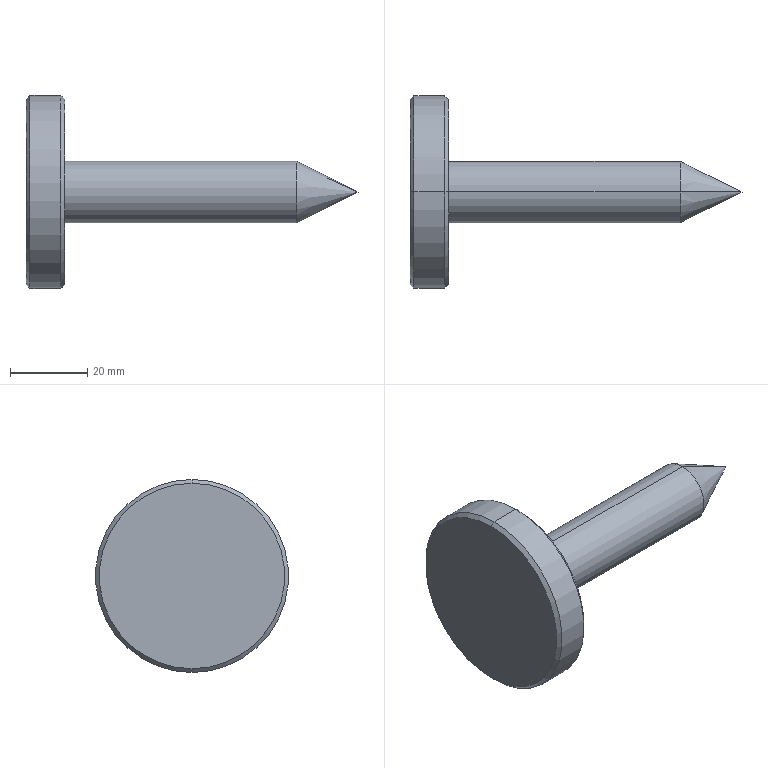Part | SolidWorks | features Chamfer 1, Extrusion 1, ICE 1, Revolution 1 | 1 solid | 12 faces | box 86 x 50 x 50 mm | volume 32616 mm3 | cone 6 | cylinder 4 | plane 2 | commonest cylinder face diameters 16 x2 50 x2
STEP:
#1=CARTESIAN_POINT('',(0.,0.,24.));
#2=VERTEX_POINT('',#1);
#3=CARTESIAN_POINT('',(0.,0.,-24.));
#4=VERTEX_POINT('',#3);
#5=CARTESIAN_POINT('',(0.,0.,0.));
#6=DIRECTION('',(-1.,0.,0.));
#7=DIRECTION('',(0.,0.,-1.));
#8=AXIS2_PLACEMENT_3D('',#5,#6,#7);
#9=CIRCLE('',#8,24.);
#10=EDGE_CURVE('',#2,#4,#9,.T.);
#11=ORIENTED_EDGE('',*,*,#10,.F.);
#12=CARTESIAN_POINT('',(1.,0.,25.));
#13=VERTEX_POINT('',#12);
#14=CARTESIAN_POINT('',(1.,0.,25.));
#15=DIRECTION('',(0.7071,0.,0.7071));
#16=VECTOR('',#15,1000.);
#17=LINE('',#14,#16);
#18=EDGE_CURVE('',#2,#13,#17,.T.);
#19=ORIENTED_EDGE('',*,*,#18,.T.);
#20=CARTESIAN_POINT('',(1.,0.,-25.));
#21=VERTEX_POINT('',#20);
#22=CARTESIAN_POINT('',(1.,0.,0.));
#23=DIRECTION('',(1.,0.,0.));
#24=DIRECTION('',(0.,0.,-1.));
#25=AXIS2_PLACEMENT_3D('',#22,#23,#24);
#26=CIRCLE('',#25,25.);
#27=EDGE_CURVE('',#21,#13,#26,.T.);
#28=ORIENTED_EDGE('',*,*,#27,.F.);
#29=CARTESIAN_POINT('',(1.,0.,-25.));
#30=DIRECTION('',(0.7071,0.,-0.7071));
#31=VECTOR('',#30,1000.);
#32=LINE('',#29,#31);
#33=EDGE_CURVE('',#4,#21,#32,.T.);
#34=ORIENTED_EDGE('',*,*,#33,.F.);
#35=EDGE_LOOP('',(#11,#19,#28,#34));
#36=FACE_OUTER_BOUND('',#35,.T.);
#37=CARTESIAN_POINT('',(1.,0.,0.));
#38=DIRECTION('',(1.,0.,0.));
#39=DIRECTION('',(0.,0.,-1.));
#40=AXIS2_PLACEMENT_3D('',#37,#38,#39);
#41=CONICAL_SURFACE('',#40,25.,0.7854);
#42=ADVANCED_FACE('',(#36),#41,.T.);
#43=CARTESIAN_POINT('',(10.,0.,-24.));
#44=VERTEX_POINT('',#43);
#45=CARTESIAN_POINT('',(10.,0.,24.));
#46=VERTEX_POINT('',#45);
#47=CARTESIAN_POINT('',(10.,0.,0.));
#48=DIRECTION('',(1.,0.,0.));
#49=DIRECTION('',(0.,0.,-1.));
#50=AXIS2_PLACEMENT_3D('',#47,#48,#49);
#51=CIRCLE('',#50,24.);
#52=EDGE_CURVE('',#44,#46,#51,.T.);
#53=ORIENTED_EDGE('',*,*,#52,.F.);
#54=CARTESIAN_POINT('',(9.,0.,-25.));
#55=VERTEX_POINT('',#54);
#56=CARTESIAN_POINT('',(10.,0.,-24.));
#57=DIRECTION('',(-0.7071,0.,-0.7071));
#58=VECTOR('',#57,1000.);
#59=LINE('',#56,#58);
#60=EDGE_CURVE('',#44,#55,#59,.T.);
#61=ORIENTED_EDGE('',*,*,#60,.T.);
#62=CARTESIAN_POINT('',(9.,0.,25.));
#63=VERTEX_POINT('',#62);
#64=CARTESIAN_POINT('',(9.,0.,0.));
#65=DIRECTION('',(-1.,0.,0.));
#66=DIRECTION('',(0.,0.,-1.));
#67=AXIS2_PLACEMENT_3D('',#64,#65,#66);
#68=CIRCLE('',#67,25.);
#69=EDGE_CURVE('',#63,#55,#68,.T.);
#70=ORIENTED_EDGE('',*,*,#69,.F.);
#71=CARTESIAN_POINT('',(10.,0.,24.));
#72=DIRECTION('',(-0.7071,0.,0.7071));
#73=VECTOR('',#72,1000.);
#74=LINE('',#71,#73);
#75=EDGE_CURVE('',#46,#63,#74,.T.);
#76=ORIENTED_EDGE('',*,*,#75,.F.);
#77=EDGE_LOOP('',(#53,#61,#70,#76));
#78=FACE_OUTER_BOUND('',#77,.T.);
#79=CARTESIAN_POINT('',(10.,0.,0.));
#80=DIRECTION('',(-1.,0.,0.));
#81=DIRECTION('',(0.,0.,1.));
#82=AXIS2_PLACEMENT_3D('',#79,#80,#81);
#83=CONICAL_SURFACE('',#82,24.,0.7854);
#84=ADVANCED_FACE('',(#78),#83,.T.);
#85=CARTESIAN_POINT('',(86.,0.,0.));
#86=VERTEX_POINT('',#85);
#87=CARTESIAN_POINT('',(70.,0.,8.));
#88=VERTEX_POINT('',#87);
#89=CARTESIAN_POINT('',(86.,0.,0.));
#90=DIRECTION('',(-0.8944,0.,0.4472));
#91=VECTOR('',#90,1000.);
#92=LINE('',#89,#91);
#93=EDGE_CURVE('',#86,#88,#92,.T.);
#94=ORIENTED_EDGE('',*,*,#93,.F.);
#95=CARTESIAN_POINT('',(70.,0.,-8.));
#96=VERTEX_POINT('',#95);
#97=CARTESIAN_POINT('',(86.,0.,0.));
#98=DIRECTION('',(-0.8944,0.,-0.4472));
#99=VECTOR('',#98,1000.);
#100=LINE('',#97,#99);
#101=EDGE_CURVE('',#86,#96,#100,.T.);
#102=ORIENTED_EDGE('',*,*,#101,.T.);
#103=CARTESIAN_POINT('',(70.,0.,0.));
#104=DIRECTION('',(1.,0.,0.));
#105=DIRECTION('',(0.,0.,-1.));
#106=AXIS2_PLACEMENT_3D('',#103,#104,#105);
#107=CIRCLE('',#106,8.);
#108=EDGE_CURVE('',#96,#88,#107,.T.);
#109=ORIENTED_EDGE('',*,*,#108,.T.);
#110=EDGE_LOOP('',(#94,#102,#109));
#111=FACE_OUTER_BOUND('',#110,.T.);
#112=CARTESIAN_POINT('',(-914.,0.,0.));
#113=DIRECTION('',(-1.,0.,0.));
#114=DIRECTION('',(0.,0.,1.));
#115=AXIS2_PLACEMENT_3D('',#112,#113,#114);
#116=CONICAL_SURFACE('',#115,500.,0.4636);
#117=ADVANCED_FACE('',(#111),#116,.T.);
#118=ORIENTED_EDGE('',*,*,#108,.F.);
#119=CARTESIAN_POINT('',(10.,0.,-8.));
#120=VERTEX_POINT('',#119);
#121=CARTESIAN_POINT('',(70.,0.,-8.));
#122=DIRECTION('',(-1.,0.,0.));
#123=VECTOR('',#122,1000.);
#124=LINE('',#121,#123);
#125=EDGE_CURVE('',#96,#120,#124,.T.);
#126=ORIENTED_EDGE('',*,*,#125,.T.);
#127=CARTESIAN_POINT('',(10.,0.,8.));
#128=VERTEX_POINT('',#127);
#129=CARTESIAN_POINT('',(10.,0.,0.));
#130=DIRECTION('',(1.,0.,0.));
#131=DIRECTION('',(0.,0.,-1.));
#132=AXIS2_PLACEMENT_3D('',#129,#130,#131);
#133=CIRCLE('',#132,8.);
#134=EDGE_CURVE('',#120,#128,#133,.T.);
#135=ORIENTED_EDGE('',*,*,#134,.T.);
#136=CARTESIAN_POINT('',(70.,0.,8.));
#137=DIRECTION('',(-1.,0.,0.));
#138=VECTOR('',#137,1000.);
#139=LINE('',#136,#138);
#140=EDGE_CURVE('',#88,#128,#139,.T.);
#141=ORIENTED_EDGE('',*,*,#140,.F.);
#142=EDGE_LOOP('',(#118,#126,#135,#141));
#143=FACE_OUTER_BOUND('',#142,.T.);
#144=CARTESIAN_POINT('',(70.,0.,0.));
#145=DIRECTION('',(-1.,0.,0.));
#146=DIRECTION('',(0.,0.,1.));
#147=AXIS2_PLACEMENT_3D('',#144,#145,#146);
#148=CYLINDRICAL_SURFACE('',#147,8.);
#149=ADVANCED_FACE('',(#143),#148,.T.);
#150=ORIENTED_EDGE('',*,*,#69,.T.);
#151=CARTESIAN_POINT('',(10.,0.,-25.));
#152=DIRECTION('',(-1.,0.,0.));
#153=VECTOR('',#152,1000.);
#154=LINE('',#151,#153);
#155=EDGE_CURVE('',#55,#21,#154,.T.);
#156=ORIENTED_EDGE('',*,*,#155,.T.);
#157=ORIENTED_EDGE('',*,*,#27,.T.);
#158=CARTESIAN_POINT('',(10.,0.,25.));
#159=DIRECTION('',(-1.,0.,0.));
#160=VECTOR('',#159,1000.);
#161=LINE('',#158,#160);
#162=EDGE_CURVE('',#63,#13,#161,.T.);
#163=ORIENTED_EDGE('',*,*,#162,.F.);
#164=EDGE_LOOP('',(#150,#156,#157,#163));
#165=FACE_OUTER_BOUND('',#164,.T.);
#166=CARTESIAN_POINT('',(10.,0.,0.));
#167=DIRECTION('',(-1.,0.,0.));
#168=DIRECTION('',(0.,0.,1.));
#169=AXIS2_PLACEMENT_3D('',#166,#167,#168);
#170=CYLINDRICAL_SURFACE('',#169,25.);
#171=ADVANCED_FACE('',(#165),#170,.T.);
#172=ORIENTED_EDGE('',*,*,#155,.F.);
#173=CARTESIAN_POINT('',(9.,0.,0.));
#174=DIRECTION('',(-1.,0.,0.));
#175=DIRECTION('',(0.,0.,-1.));
#176=AXIS2_PLACEMENT_3D('',#173,#174,#175);
#177=CIRCLE('',#176,25.);
#178=EDGE_CURVE('',#55,#63,#177,.T.);
#179=ORIENTED_EDGE('',*,*,#178,.T.);
#180=ORIENTED_EDGE('',*,*,#162,.T.);
#181=CARTESIAN_POINT('',(1.,0.,0.));
#182=DIRECTION('',(1.,0.,0.));
#183=DIRECTION('',(0.,0.,-1.));
#184=AXIS2_PLACEMENT_3D('',#181,#182,#183);
#185=CIRCLE('',#184,25.);
#186=EDGE_CURVE('',#13,#21,#185,.T.);
#187=ORIENTED_EDGE('',*,*,#186,.T.);
#188=EDGE_LOOP('',(#172,#179,#180,#187));
#189=FACE_OUTER_BOUND('',#188,.T.);
#190=CARTESIAN_POINT('',(10.,0.,0.));
#191=DIRECTION('',(-1.,0.,0.));
#192=DIRECTION('',(0.,0.,1.));
#193=AXIS2_PLACEMENT_3D('',#190,#191,#192);
#194=CYLINDRICAL_SURFACE('',#193,25.);
#195=ADVANCED_FACE('',(#189),#194,.T.);
#196=CARTESIAN_POINT('',(10.,0.,0.));
#197=DIRECTION('',(1.,0.,0.));
#198=DIRECTION('',(0.,0.,-1.));
#199=AXIS2_PLACEMENT_3D('',#196,#197,#198);
#200=CIRCLE('',#199,24.);
#201=EDGE_CURVE('',#46,#44,#200,.T.);
#202=ORIENTED_EDGE('',*,*,#201,.T.);
#203=ORIENTED_EDGE('',*,*,#52,.T.);
#204=EDGE_LOOP('',(#202,#203));
#205=FACE_OUTER_BOUND('',#204,.T.);
#206=CARTESIAN_POINT('',(10.,0.,0.));
#207=DIRECTION('',(1.,0.,0.));
#208=DIRECTION('',(0.,0.,-1.));
#209=AXIS2_PLACEMENT_3D('',#206,#207,#208);
#210=CIRCLE('',#209,8.);
#211=EDGE_CURVE('',#128,#120,#210,.T.);
#212=ORIENTED_EDGE('',*,*,#211,.F.);
#213=ORIENTED_EDGE('',*,*,#134,.F.);
#214=EDGE_LOOP('',(#212,#213));
#215=FACE_BOUND('',#214,.T.);
#216=CARTESIAN_POINT('',(10.,0.,0.));
#217=DIRECTION('',(1.,0.,0.));
#218=DIRECTION('',(0.,0.,-1.));
#219=AXIS2_PLACEMENT_3D('',#216,#217,#218);
#220=PLANE('',#219);
#221=ADVANCED_FACE('',(#205,#215),#220,.T.);
#222=CARTESIAN_POINT('',(0.,0.,0.));
#223=DIRECTION('',(-1.,0.,0.));
#224=DIRECTION('',(0.,0.,-1.));
#225=AXIS2_PLACEMENT_3D('',#222,#223,#224);
#226=CIRCLE('',#225,24.);
#227=EDGE_CURVE('',#4,#2,#226,.T.);
#228=ORIENTED_EDGE('',*,*,#227,.T.);
#229=ORIENTED_EDGE('',*,*,#10,.T.);
#230=EDGE_LOOP('',(#228,#229));
#231=FACE_OUTER_BOUND('',#230,.T.);
#232=CARTESIAN_POINT('',(0.,0.,0.));
#233=DIRECTION('',(1.,0.,0.));
#234=DIRECTION('',(0.,0.,-1.));
#235=AXIS2_PLACEMENT_3D('',#232,#233,#234);
#236=PLANE('',#235);
#237=ADVANCED_FACE('',(#231),#236,.F.);
#238=ORIENTED_EDGE('',*,*,#125,.F.);
#239=CARTESIAN_POINT('',(70.,0.,0.));
#240=DIRECTION('',(1.,0.,0.));
#241=DIRECTION('',(0.,0.,-1.));
#242=AXIS2_PLACEMENT_3D('',#239,#240,#241);
#243=CIRCLE('',#242,8.);
#244=EDGE_CURVE('',#88,#96,#243,.T.);
#245=ORIENTED_EDGE('',*,*,#244,.F.);
#246=ORIENTED_EDGE('',*,*,#140,.T.);
#247=ORIENTED_EDGE('',*,*,#211,.T.);
#248=EDGE_LOOP('',(#238,#245,#246,#247));
#249=FACE_OUTER_BOUND('',#248,.T.);
#250=CARTESIAN_POINT('',(70.,0.,0.));
#251=DIRECTION('',(-1.,0.,0.));
#252=DIRECTION('',(0.,0.,1.));
#253=AXIS2_PLACEMENT_3D('',#250,#251,#252);
#254=CYLINDRICAL_SURFACE('',#253,8.);
#255=ADVANCED_FACE('',(#249),#254,.T.);
#256=ORIENTED_EDGE('',*,*,#101,.F.);
#257=ORIENTED_EDGE('',*,*,#93,.T.);
#258=ORIENTED_EDGE('',*,*,#244,.T.);
#259=EDGE_LOOP('',(#256,#257,#258));
#260=FACE_OUTER_BOUND('',#259,.T.);
#261=CARTESIAN_POINT('',(-914.,0.,0.));
#262=DIRECTION('',(-1.,0.,0.));
#263=DIRECTION('',(0.,0.,1.));
#264=AXIS2_PLACEMENT_3D('',#261,#262,#263);
#265=CONICAL_SURFACE('',#264,500.,0.4636);
#266=ADVANCED_FACE('',(#260),#265,.T.);
#267=ORIENTED_EDGE('',*,*,#60,.F.);
#268=ORIENTED_EDGE('',*,*,#201,.F.);
#269=ORIENTED_EDGE('',*,*,#75,.T.);
#270=ORIENTED_EDGE('',*,*,#178,.F.);
#271=EDGE_LOOP('',(#267,#268,#269,#270));
#272=FACE_OUTER_BOUND('',#271,.T.);
#273=CARTESIAN_POINT('',(10.,0.,0.));
#274=DIRECTION('',(-1.,0.,0.));
#275=DIRECTION('',(0.,0.,1.));
#276=AXIS2_PLACEMENT_3D('',#273,#274,#275);
#277=CONICAL_SURFACE('',#276,24.,0.7854);
#278=ADVANCED_FACE('',(#272),#277,.T.);
#279=ORIENTED_EDGE('',*,*,#18,.F.);
#280=ORIENTED_EDGE('',*,*,#227,.F.);
#281=ORIENTED_EDGE('',*,*,#33,.T.);
#282=ORIENTED_EDGE('',*,*,#186,.F.);
#283=EDGE_LOOP('',(#279,#280,#281,#282));
#284=FACE_OUTER_BOUND('',#283,.T.);
#285=CARTESIAN_POINT('',(1.,0.,0.));
#286=DIRECTION('',(1.,0.,0.));
#287=DIRECTION('',(0.,0.,-1.));
#288=AXIS2_PLACEMENT_3D('',#285,#286,#287);
#289=CONICAL_SURFACE('',#288,25.,0.7854);
#290=ADVANCED_FACE('',(#284),#289,.T.);
#291=CLOSED_SHELL('',(#42,#84,#117,#149,#171,#195,#221,#237,#255,#266,#278,#290));
#292=MANIFOLD_SOLID_BREP('',#291);
#293=CARTESIAN_POINT('',(0.,0.,0.));
#294=DIRECTION('',(0.,0.,1.));
#295=DIRECTION('',(1.,0.,0.));
#296=AXIS2_PLACEMENT_3D('',#293,#294,#295);
#297=(LENGTH_UNIT()NAMED_UNIT(*)SI_UNIT(.MILLI.,.METRE.));
#298=UNCERTAINTY_MEASURE_WITH_UNIT(LENGTH_MEASURE(0.00001),#297,'','');
#299=(NAMED_UNIT(*)PLANE_ANGLE_UNIT()SI_UNIT($,.RADIAN.));
#300=(NAMED_UNIT(*)SI_UNIT($,.STERADIAN.)SOLID_ANGLE_UNIT());
#301=(GEOMETRIC_REPRESENTATION_CONTEXT(3)GLOBAL_UNCERTAINTY_ASSIGNED_CONTEXT((#298))GLOBAL_UNIT_ASSIGNED_CONTEXT((#297,#299,#300))REPRESENTATION_CONTEXT('',''));
#302=ADVANCED_BREP_SHAPE_REPRESENTATION('',(#292,#296),#301);